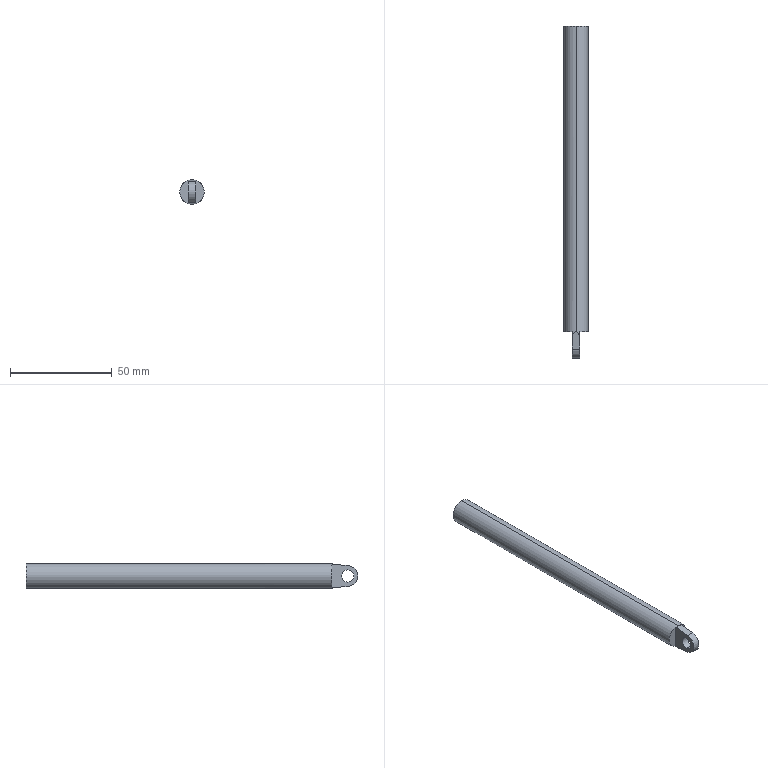Part | SolidWorks | features ICE 2, Extrusion 1, Shell 1 | 1 solid | 15 faces | box 12 x 163 x 12 mm | volume 9872 mm3 | plane 8 | cylinder 7 | commonest cylinder face diameters 6 x2 8 x2 12 x2 10 x1
STEP:
#1=CARTESIAN_POINT('',(1.75,-8.,3.));
#2=VERTEX_POINT('',#1);
#3=CARTESIAN_POINT('',(1.75,-8.,-3.));
#4=VERTEX_POINT('',#3);
#5=CARTESIAN_POINT('',(1.75,-8.,0.));
#6=DIRECTION('',(1.,0.,0.));
#7=DIRECTION('',(0.,0.,-1.));
#8=AXIS2_PLACEMENT_3D('',#5,#6,#7);
#9=CIRCLE('',#8,3.);
#10=EDGE_CURVE('',#2,#4,#9,.T.);
#11=ORIENTED_EDGE('',*,*,#10,.T.);
#12=CARTESIAN_POINT('',(-1.75,-8.,-3.));
#13=VERTEX_POINT('',#12);
#14=CARTESIAN_POINT('',(1.75,-8.,-3.));
#15=DIRECTION('',(-1.,0.,0.));
#16=VECTOR('',#15,1000.);
#17=LINE('',#14,#16);
#18=EDGE_CURVE('',#4,#13,#17,.T.);
#19=ORIENTED_EDGE('',*,*,#18,.T.);
#20=CARTESIAN_POINT('',(-1.75,-8.,3.));
#21=VERTEX_POINT('',#20);
#22=CARTESIAN_POINT('',(-1.75,-8.,0.));
#23=DIRECTION('',(1.,0.,0.));
#24=DIRECTION('',(0.,0.,-1.));
#25=AXIS2_PLACEMENT_3D('',#22,#23,#24);
#26=CIRCLE('',#25,3.);
#27=EDGE_CURVE('',#21,#13,#26,.T.);
#28=ORIENTED_EDGE('',*,*,#27,.F.);
#29=CARTESIAN_POINT('',(1.75,-8.,3.));
#30=DIRECTION('',(-1.,0.,0.));
#31=VECTOR('',#30,1000.);
#32=LINE('',#29,#31);
#33=EDGE_CURVE('',#2,#21,#32,.T.);
#34=ORIENTED_EDGE('',*,*,#33,.F.);
#35=EDGE_LOOP('',(#11,#19,#28,#34));
#36=FACE_OUTER_BOUND('',#35,.T.);
#37=CARTESIAN_POINT('',(1.75,-8.,0.));
#38=DIRECTION('',(-1.,0.,0.));
#39=DIRECTION('',(0.,0.,1.));
#40=AXIS2_PLACEMENT_3D('',#37,#38,#39);
#41=CYLINDRICAL_SURFACE('',#40,3.);
#42=ADVANCED_FACE('',(#36),#41,.F.);
#43=CARTESIAN_POINT('',(0.,150.,-4.));
#44=VERTEX_POINT('',#43);
#45=CARTESIAN_POINT('',(0.,150.,4.));
#46=VERTEX_POINT('',#45);
#47=CARTESIAN_POINT('',(0.,150.,0.));
#48=DIRECTION('',(0.,1.,0.));
#49=DIRECTION('',(0.,0.,1.));
#50=AXIS2_PLACEMENT_3D('',#47,#48,#49);
#51=CIRCLE('',#50,4.);
#52=EDGE_CURVE('',#44,#46,#51,.T.);
#53=ORIENTED_EDGE('',*,*,#52,.T.);
#54=CARTESIAN_POINT('',(0.,2.,4.));
#55=VERTEX_POINT('',#54);
#56=CARTESIAN_POINT('',(0.,150.,4.));
#57=DIRECTION('',(0.,-1.,0.));
#58=VECTOR('',#57,1000.);
#59=LINE('',#56,#58);
#60=EDGE_CURVE('',#46,#55,#59,.T.);
#61=ORIENTED_EDGE('',*,*,#60,.T.);
#62=CARTESIAN_POINT('',(0.,2.,-4.));
#63=VERTEX_POINT('',#62);
#64=CARTESIAN_POINT('',(0.,2.,0.));
#65=DIRECTION('',(0.,1.,0.));
#66=DIRECTION('',(0.,0.,1.));
#67=AXIS2_PLACEMENT_3D('',#64,#65,#66);
#68=CIRCLE('',#67,4.);
#69=EDGE_CURVE('',#63,#55,#68,.T.);
#70=ORIENTED_EDGE('',*,*,#69,.F.);
#71=CARTESIAN_POINT('',(0.,150.,-4.));
#72=DIRECTION('',(0.,-1.,0.));
#73=VECTOR('',#72,1000.);
#74=LINE('',#71,#73);
#75=EDGE_CURVE('',#44,#63,#74,.T.);
#76=ORIENTED_EDGE('',*,*,#75,.F.);
#77=EDGE_LOOP('',(#53,#61,#70,#76));
#78=FACE_OUTER_BOUND('',#77,.T.);
#79=CARTESIAN_POINT('',(0.,150.,0.));
#80=DIRECTION('',(0.,-1.,0.));
#81=DIRECTION('',(0.,0.,-1.));
#82=AXIS2_PLACEMENT_3D('',#79,#80,#81);
#83=CYLINDRICAL_SURFACE('',#82,4.);
#84=ADVANCED_FACE('',(#78),#83,.F.);
#85=CARTESIAN_POINT('',(0.,150.,6.));
#86=VERTEX_POINT('',#85);
#87=CARTESIAN_POINT('',(0.,150.,-6.));
#88=VERTEX_POINT('',#87);
#89=CARTESIAN_POINT('',(0.,150.,0.));
#90=DIRECTION('',(0.,1.,0.));
#91=DIRECTION('',(0.,0.,1.));
#92=AXIS2_PLACEMENT_3D('',#89,#90,#91);
#93=CIRCLE('',#92,6.);
#94=EDGE_CURVE('',#86,#88,#93,.T.);
#95=ORIENTED_EDGE('',*,*,#94,.F.);
#96=CARTESIAN_POINT('',(0.,0.,6.));
#97=VERTEX_POINT('',#96);
#98=CARTESIAN_POINT('',(0.,150.,6.));
#99=DIRECTION('',(0.,-1.,0.));
#100=VECTOR('',#99,1000.);
#101=LINE('',#98,#100);
#102=EDGE_CURVE('',#86,#97,#101,.T.);
#103=ORIENTED_EDGE('',*,*,#102,.T.);
#104=CARTESIAN_POINT('',(1.75,-2.165,5.739));
#105=VERTEX_POINT('',#104);
#106=CARTESIAN_POINT('',(1.75,-2.165,5.739));
#107=CARTESIAN_POINT('',(1.182,-0.7271,5.912));
#108=CARTESIAN_POINT('',(0.5941,0.,6.));
#109=CARTESIAN_POINT('',(0.,0.,6.));
#110=(BOUNDED_CURVE()B_SPLINE_CURVE(3,(#106,#107,#108,#109),.UNSPECIFIED.,.F.,.F.)B_SPLINE_CURVE_WITH_KNOTS((4,4),(5.987,6.283),.UNSPECIFIED.)CURVE()GEOMETRIC_REPRESENTATION_ITEM()RATIONAL_B_SPLINE_CURVE((1.,0.9927,0.9927,1.))REPRESENTATION_ITEM(''));
#111=EDGE_CURVE('',#105,#97,#110,.T.);
#112=ORIENTED_EDGE('',*,*,#111,.F.);
#113=CARTESIAN_POINT('',(1.75,0.,5.739));
#114=VERTEX_POINT('',#113);
#115=CARTESIAN_POINT('',(1.75,-10.,5.739));
#116=DIRECTION('',(0.,1.,0.));
#117=VECTOR('',#116,1000.);
#118=LINE('',#115,#117);
#119=EDGE_CURVE('',#105,#114,#118,.T.);
#120=ORIENTED_EDGE('',*,*,#119,.T.);
#121=CARTESIAN_POINT('',(1.75,0.,-5.739));
#122=VERTEX_POINT('',#121);
#123=CARTESIAN_POINT('',(0.,0.,0.));
#124=DIRECTION('',(0.,1.,0.));
#125=DIRECTION('',(0.,0.,1.));
#126=AXIS2_PLACEMENT_3D('',#123,#124,#125);
#127=CIRCLE('',#126,6.);
#128=EDGE_CURVE('',#114,#122,#127,.T.);
#129=ORIENTED_EDGE('',*,*,#128,.T.);
#130=CARTESIAN_POINT('',(1.75,-2.165,-5.739));
#131=VERTEX_POINT('',#130);
#132=CARTESIAN_POINT('',(1.75,-10.,-5.739));
#133=DIRECTION('',(0.,-1.,0.));
#134=VECTOR('',#133,1000.);
#135=LINE('',#132,#134);
#136=EDGE_CURVE('',#122,#131,#135,.T.);
#137=ORIENTED_EDGE('',*,*,#136,.T.);
#138=CARTESIAN_POINT('',(0.,0.,-6.));
#139=VERTEX_POINT('',#138);
#140=CARTESIAN_POINT('',(0.,0.,-6.));
#141=CARTESIAN_POINT('',(0.5941,0.,-6.));
#142=CARTESIAN_POINT('',(1.182,-0.7271,-5.912));
#143=CARTESIAN_POINT('',(1.75,-2.165,-5.739));
#144=(BOUNDED_CURVE()B_SPLINE_CURVE(3,(#140,#141,#142,#143),.UNSPECIFIED.,.F.,.F.)B_SPLINE_CURVE_WITH_KNOTS((4,4),(0.,0.296),.UNSPECIFIED.)CURVE()GEOMETRIC_REPRESENTATION_ITEM()RATIONAL_B_SPLINE_CURVE((1.,0.9927,0.9927,1.))REPRESENTATION_ITEM(''));
#145=EDGE_CURVE('',#139,#131,#144,.T.);
#146=ORIENTED_EDGE('',*,*,#145,.F.);
#147=CARTESIAN_POINT('',(0.,150.,-6.));
#148=DIRECTION('',(0.,-1.,0.));
#149=VECTOR('',#148,1000.);
#150=LINE('',#147,#149);
#151=EDGE_CURVE('',#88,#139,#150,.T.);
#152=ORIENTED_EDGE('',*,*,#151,.F.);
#153=EDGE_LOOP('',(#95,#103,#112,#120,#129,#137,#146,#152));
#154=FACE_OUTER_BOUND('',#153,.T.);
#155=CARTESIAN_POINT('',(0.,150.,0.));
#156=DIRECTION('',(0.,-1.,0.));
#157=DIRECTION('',(0.,0.,-1.));
#158=AXIS2_PLACEMENT_3D('',#155,#156,#157);
#159=CYLINDRICAL_SURFACE('',#158,6.);
#160=ADVANCED_FACE('',(#154),#159,.T.);
#161=CARTESIAN_POINT('',(1.75,-8.598,4.964));
#162=VERTEX_POINT('',#161);
#163=CARTESIAN_POINT('',(1.75,0.,6.));
#164=DIRECTION('',(0.,-0.9928,-0.1196));
#165=VECTOR('',#164,1000.);
#166=LINE('',#163,#165);
#167=EDGE_CURVE('',#105,#162,#166,.T.);
#168=ORIENTED_EDGE('',*,*,#167,.F.);
#169=ORIENTED_EDGE('',*,*,#111,.T.);
#170=CARTESIAN_POINT('',(-1.75,-2.165,5.739));
#171=VERTEX_POINT('',#170);
#172=CARTESIAN_POINT('',(0.,0.,6.));
#173=CARTESIAN_POINT('',(-0.5941,0.,6.));
#174=CARTESIAN_POINT('',(-1.182,-0.7271,5.912));
#175=CARTESIAN_POINT('',(-1.75,-2.165,5.739));
#176=(BOUNDED_CURVE()B_SPLINE_CURVE(3,(#172,#173,#174,#175),.UNSPECIFIED.,.F.,.F.)B_SPLINE_CURVE_WITH_KNOTS((4,4),(0.,0.296),.UNSPECIFIED.)CURVE()GEOMETRIC_REPRESENTATION_ITEM()RATIONAL_B_SPLINE_CURVE((1.,0.9927,0.9927,1.))REPRESENTATION_ITEM(''));
#177=EDGE_CURVE('',#97,#171,#176,.T.);
#178=ORIENTED_EDGE('',*,*,#177,.T.);
#179=CARTESIAN_POINT('',(-1.75,-8.598,4.964));
#180=VERTEX_POINT('',#179);
#181=CARTESIAN_POINT('',(-1.75,0.,6.));
#182=DIRECTION('',(0.,-0.9928,-0.1196));
#183=VECTOR('',#182,1000.);
#184=LINE('',#181,#183);
#185=EDGE_CURVE('',#171,#180,#184,.T.);
#186=ORIENTED_EDGE('',*,*,#185,.T.);
#187=CARTESIAN_POINT('',(1.75,-8.598,4.964));
#188=DIRECTION('',(-1.,0.,0.));
#189=VECTOR('',#188,1000.);
#190=LINE('',#187,#189);
#191=EDGE_CURVE('',#162,#180,#190,.T.);
#192=ORIENTED_EDGE('',*,*,#191,.F.);
#193=EDGE_LOOP('',(#168,#169,#178,#186,#192));
#194=FACE_OUTER_BOUND('',#193,.T.);
#195=CARTESIAN_POINT('',(1.75,0.,6.));
#196=DIRECTION('',(0.,0.1196,-0.9928));
#197=DIRECTION('',(0.,0.9928,0.1196));
#198=AXIS2_PLACEMENT_3D('',#195,#196,#197);
#199=PLANE('',#198);
#200=ADVANCED_FACE('',(#194),#199,.F.);
#201=CARTESIAN_POINT('',(-1.75,-2.165,-5.739));
#202=VERTEX_POINT('',#201);
#203=CARTESIAN_POINT('',(-1.75,-2.165,-5.739));
#204=CARTESIAN_POINT('',(-1.182,-0.7271,-5.912));
#205=CARTESIAN_POINT('',(-0.5941,0.,-6.));
#206=CARTESIAN_POINT('',(0.,0.,-6.));
#207=(BOUNDED_CURVE()B_SPLINE_CURVE(3,(#203,#204,#205,#206),.UNSPECIFIED.,.F.,.F.)B_SPLINE_CURVE_WITH_KNOTS((4,4),(5.987,6.283),.UNSPECIFIED.)CURVE()GEOMETRIC_REPRESENTATION_ITEM()RATIONAL_B_SPLINE_CURVE((1.,0.9927,0.9927,1.))REPRESENTATION_ITEM(''));
#208=EDGE_CURVE('',#202,#139,#207,.T.);
#209=ORIENTED_EDGE('',*,*,#208,.T.);
#210=ORIENTED_EDGE('',*,*,#145,.T.);
#211=CARTESIAN_POINT('',(1.75,-8.598,-4.964));
#212=VERTEX_POINT('',#211);
#213=CARTESIAN_POINT('',(1.75,0.,-6.));
#214=DIRECTION('',(0.,0.9928,-0.1196));
#215=VECTOR('',#214,1000.);
#216=LINE('',#213,#215);
#217=EDGE_CURVE('',#212,#131,#216,.T.);
#218=ORIENTED_EDGE('',*,*,#217,.F.);
#219=CARTESIAN_POINT('',(-1.75,-8.598,-4.964));
#220=VERTEX_POINT('',#219);
#221=CARTESIAN_POINT('',(1.75,-8.598,-4.964));
#222=DIRECTION('',(-1.,0.,0.));
#223=VECTOR('',#222,1000.);
#224=LINE('',#221,#223);
#225=EDGE_CURVE('',#212,#220,#224,.T.);
#226=ORIENTED_EDGE('',*,*,#225,.T.);
#227=CARTESIAN_POINT('',(-1.75,0.,-6.));
#228=DIRECTION('',(0.,0.9928,-0.1196));
#229=VECTOR('',#228,1000.);
#230=LINE('',#227,#229);
#231=EDGE_CURVE('',#220,#202,#230,.T.);
#232=ORIENTED_EDGE('',*,*,#231,.T.);
#233=EDGE_LOOP('',(#209,#210,#218,#226,#232));
#234=FACE_OUTER_BOUND('',#233,.T.);
#235=CARTESIAN_POINT('',(1.75,0.,-6.));
#236=DIRECTION('',(0.,0.1196,0.9928));
#237=DIRECTION('',(0.,-0.9928,0.1196));
#238=AXIS2_PLACEMENT_3D('',#235,#236,#237);
#239=PLANE('',#238);
#240=ADVANCED_FACE('',(#234),#239,.F.);
#241=CARTESIAN_POINT('',(1.75,0.,6.));
#242=DIRECTION('',(0.,0.,1.));
#243=VECTOR('',#242,1000.);
#244=LINE('',#241,#243);
#245=EDGE_CURVE('',#122,#114,#244,.T.);
#246=ORIENTED_EDGE('',*,*,#245,.F.);
#247=ORIENTED_EDGE('',*,*,#128,.F.);
#248=EDGE_LOOP('',(#246,#247));
#249=FACE_OUTER_BOUND('',#248,.T.);
#250=CARTESIAN_POINT('',(0.,0.,0.));
#251=DIRECTION('',(0.,1.,0.));
#252=DIRECTION('',(0.,0.,1.));
#253=AXIS2_PLACEMENT_3D('',#250,#251,#252);
#254=PLANE('',#253);
#255=ADVANCED_FACE('',(#249),#254,.F.);
#256=ORIENTED_EDGE('',*,*,#102,.F.);
#257=CARTESIAN_POINT('',(0.,150.,0.));
#258=DIRECTION('',(0.,1.,0.));
#259=DIRECTION('',(0.,0.,1.));
#260=AXIS2_PLACEMENT_3D('',#257,#258,#259);
#261=CIRCLE('',#260,6.);
#262=EDGE_CURVE('',#88,#86,#261,.T.);
#263=ORIENTED_EDGE('',*,*,#262,.F.);
#264=ORIENTED_EDGE('',*,*,#151,.T.);
#265=ORIENTED_EDGE('',*,*,#208,.F.);
#266=CARTESIAN_POINT('',(-1.75,0.,-5.739));
#267=VERTEX_POINT('',#266);
#268=CARTESIAN_POINT('',(-1.75,-10.,-5.739));
#269=DIRECTION('',(0.,-1.,0.));
#270=VECTOR('',#269,1000.);
#271=LINE('',#268,#270);
#272=EDGE_CURVE('',#267,#202,#271,.T.);
#273=ORIENTED_EDGE('',*,*,#272,.F.);
#274=CARTESIAN_POINT('',(-1.75,0.,5.739));
#275=VERTEX_POINT('',#274);
#276=CARTESIAN_POINT('',(0.,0.,0.));
#277=DIRECTION('',(0.,1.,0.));
#278=DIRECTION('',(0.,0.,1.));
#279=AXIS2_PLACEMENT_3D('',#276,#277,#278);
#280=CIRCLE('',#279,6.);
#281=EDGE_CURVE('',#267,#275,#280,.T.);
#282=ORIENTED_EDGE('',*,*,#281,.T.);
#283=CARTESIAN_POINT('',(-1.75,-10.,5.739));
#284=DIRECTION('',(0.,1.,0.));
#285=VECTOR('',#284,1000.);
#286=LINE('',#283,#285);
#287=EDGE_CURVE('',#171,#275,#286,.T.);
#288=ORIENTED_EDGE('',*,*,#287,.F.);
#289=ORIENTED_EDGE('',*,*,#177,.F.);
#290=EDGE_LOOP('',(#256,#263,#264,#265,#273,#282,#288,#289));
#291=FACE_OUTER_BOUND('',#290,.T.);
#292=CARTESIAN_POINT('',(0.,150.,0.));
#293=DIRECTION('',(0.,-1.,0.));
#294=DIRECTION('',(0.,0.,-1.));
#295=AXIS2_PLACEMENT_3D('',#292,#293,#294);
#296=CYLINDRICAL_SURFACE('',#295,6.);
#297=ADVANCED_FACE('',(#291),#296,.T.);
#298=ORIENTED_EDGE('',*,*,#52,.F.);
#299=CARTESIAN_POINT('',(0.,150.,0.));
#300=DIRECTION('',(0.,1.,0.));
#301=DIRECTION('',(0.,0.,1.));
#302=AXIS2_PLACEMENT_3D('',#299,#300,#301);
#303=CIRCLE('',#302,4.);
#304=EDGE_CURVE('',#46,#44,#303,.T.);
#305=ORIENTED_EDGE('',*,*,#304,.F.);
#306=EDGE_LOOP('',(#298,#305));
#307=FACE_BOUND('',#306,.T.);
#308=ORIENTED_EDGE('',*,*,#262,.T.);
#309=ORIENTED_EDGE('',*,*,#94,.T.);
#310=EDGE_LOOP('',(#308,#309));
#311=FACE_OUTER_BOUND('',#310,.T.);
#312=CARTESIAN_POINT('',(0.,150.,0.));
#313=DIRECTION('',(0.,1.,0.));
#314=DIRECTION('',(0.,0.,1.));
#315=AXIS2_PLACEMENT_3D('',#312,#313,#314);
#316=PLANE('',#315);
#317=ADVANCED_FACE('',(#307,#311),#316,.T.);
#318=ORIENTED_EDGE('',*,*,#281,.F.);
#319=CARTESIAN_POINT('',(-1.75,0.,6.));
#320=DIRECTION('',(0.,0.,1.));
#321=VECTOR('',#320,1000.);
#322=LINE('',#319,#321);
#323=EDGE_CURVE('',#267,#275,#322,.T.);
#324=ORIENTED_EDGE('',*,*,#323,.T.);
#325=EDGE_LOOP('',(#318,#324));
#326=FACE_OUTER_BOUND('',#325,.T.);
#327=CARTESIAN_POINT('',(0.,0.,0.));
#328=DIRECTION('',(0.,1.,0.));
#329=DIRECTION('',(0.,0.,1.));
#330=AXIS2_PLACEMENT_3D('',#327,#328,#329);
#331=PLANE('',#330);
#332=ADVANCED_FACE('',(#326),#331,.F.);
#333=ORIENTED_EDGE('',*,*,#60,.F.);
#334=ORIENTED_EDGE('',*,*,#304,.T.);
#335=ORIENTED_EDGE('',*,*,#75,.T.);
#336=CARTESIAN_POINT('',(0.,2.,0.));
#337=DIRECTION('',(0.,1.,0.));
#338=DIRECTION('',(0.,0.,1.));
#339=AXIS2_PLACEMENT_3D('',#336,#337,#338);
#340=CIRCLE('',#339,4.);
#341=EDGE_CURVE('',#55,#63,#340,.T.);
#342=ORIENTED_EDGE('',*,*,#341,.F.);
#343=EDGE_LOOP('',(#333,#334,#335,#342));
#344=FACE_OUTER_BOUND('',#343,.T.);
#345=CARTESIAN_POINT('',(0.,150.,0.));
#346=DIRECTION('',(0.,-1.,0.));
#347=DIRECTION('',(0.,0.,-1.));
#348=AXIS2_PLACEMENT_3D('',#345,#346,#347);
#349=CYLINDRICAL_SURFACE('',#348,4.);
#350=ADVANCED_FACE('',(#344),#349,.F.);
#351=ORIENTED_EDGE('',*,*,#69,.T.);
#352=ORIENTED_EDGE('',*,*,#341,.T.);
#353=EDGE_LOOP('',(#351,#352));
#354=FACE_OUTER_BOUND('',#353,.T.);
#355=CARTESIAN_POINT('',(0.,2.,0.));
#356=DIRECTION('',(0.,1.,0.));
#357=DIRECTION('',(0.,0.,1.));
#358=AXIS2_PLACEMENT_3D('',#355,#356,#357);
#359=PLANE('',#358);
#360=ADVANCED_FACE('',(#354),#359,.T.);
#361=ORIENTED_EDGE('',*,*,#136,.F.);
#362=ORIENTED_EDGE('',*,*,#245,.T.);
#363=ORIENTED_EDGE('',*,*,#119,.F.);
#364=ORIENTED_EDGE('',*,*,#167,.T.);
#365=CARTESIAN_POINT('',(1.75,-8.,0.));
#366=DIRECTION('',(1.,0.,0.));
#367=DIRECTION('',(0.,0.,-1.));
#368=AXIS2_PLACEMENT_3D('',#365,#366,#367);
#369=CIRCLE('',#368,5.);
#370=EDGE_CURVE('',#162,#212,#369,.T.);
#371=ORIENTED_EDGE('',*,*,#370,.T.);
#372=ORIENTED_EDGE('',*,*,#217,.T.);
#373=EDGE_LOOP('',(#361,#362,#363,#364,#371,#372));
#374=FACE_OUTER_BOUND('',#373,.T.);
#375=ORIENTED_EDGE('',*,*,#10,.F.);
#376=CARTESIAN_POINT('',(1.75,-8.,0.));
#377=DIRECTION('',(1.,0.,0.));
#378=DIRECTION('',(0.,0.,-1.));
#379=AXIS2_PLACEMENT_3D('',#376,#377,#378);
#380=CIRCLE('',#379,3.);
#381=EDGE_CURVE('',#4,#2,#380,.T.);
#382=ORIENTED_EDGE('',*,*,#381,.F.);
#383=EDGE_LOOP('',(#375,#382));
#384=FACE_BOUND('',#383,.T.);
#385=CARTESIAN_POINT('',(1.75,-8.,0.));
#386=DIRECTION('',(1.,0.,0.));
#387=DIRECTION('',(0.,0.,-1.));
#388=AXIS2_PLACEMENT_3D('',#385,#386,#387);
#389=PLANE('',#388);
#390=ADVANCED_FACE('',(#374,#384),#389,.T.);
#391=ORIENTED_EDGE('',*,*,#323,.F.);
#392=ORIENTED_EDGE('',*,*,#272,.T.);
#393=ORIENTED_EDGE('',*,*,#231,.F.);
#394=CARTESIAN_POINT('',(-1.75,-8.,0.));
#395=DIRECTION('',(1.,0.,0.));
#396=DIRECTION('',(0.,0.,-1.));
#397=AXIS2_PLACEMENT_3D('',#394,#395,#396);
#398=CIRCLE('',#397,5.);
#399=EDGE_CURVE('',#180,#220,#398,.T.);
#400=ORIENTED_EDGE('',*,*,#399,.F.);
#401=ORIENTED_EDGE('',*,*,#185,.F.);
#402=ORIENTED_EDGE('',*,*,#287,.T.);
#403=EDGE_LOOP('',(#391,#392,#393,#400,#401,#402));
#404=FACE_OUTER_BOUND('',#403,.T.);
#405=ORIENTED_EDGE('',*,*,#27,.T.);
#406=CARTESIAN_POINT('',(-1.75,-8.,0.));
#407=DIRECTION('',(1.,0.,0.));
#408=DIRECTION('',(0.,0.,-1.));
#409=AXIS2_PLACEMENT_3D('',#406,#407,#408);
#410=CIRCLE('',#409,3.);
#411=EDGE_CURVE('',#13,#21,#410,.T.);
#412=ORIENTED_EDGE('',*,*,#411,.T.);
#413=EDGE_LOOP('',(#405,#412));
#414=FACE_BOUND('',#413,.T.);
#415=CARTESIAN_POINT('',(-1.75,-8.,0.));
#416=DIRECTION('',(1.,0.,0.));
#417=DIRECTION('',(0.,0.,-1.));
#418=AXIS2_PLACEMENT_3D('',#415,#416,#417);
#419=PLANE('',#418);
#420=ADVANCED_FACE('',(#404,#414),#419,.F.);
#421=ORIENTED_EDGE('',*,*,#399,.T.);
#422=ORIENTED_EDGE('',*,*,#225,.F.);
#423=ORIENTED_EDGE('',*,*,#370,.F.);
#424=ORIENTED_EDGE('',*,*,#191,.T.);
#425=EDGE_LOOP('',(#421,#422,#423,#424));
#426=FACE_OUTER_BOUND('',#425,.T.);
#427=CARTESIAN_POINT('',(1.75,-8.,0.));
#428=DIRECTION('',(-1.,0.,0.));
#429=DIRECTION('',(0.,0.,1.));
#430=AXIS2_PLACEMENT_3D('',#427,#428,#429);
#431=CYLINDRICAL_SURFACE('',#430,5.);
#432=ADVANCED_FACE('',(#426),#431,.T.);
#433=ORIENTED_EDGE('',*,*,#18,.F.);
#434=ORIENTED_EDGE('',*,*,#381,.T.);
#435=ORIENTED_EDGE('',*,*,#33,.T.);
#436=ORIENTED_EDGE('',*,*,#411,.F.);
#437=EDGE_LOOP('',(#433,#434,#435,#436));
#438=FACE_OUTER_BOUND('',#437,.T.);
#439=CARTESIAN_POINT('',(1.75,-8.,0.));
#440=DIRECTION('',(-1.,0.,0.));
#441=DIRECTION('',(0.,0.,1.));
#442=AXIS2_PLACEMENT_3D('',#439,#440,#441);
#443=CYLINDRICAL_SURFACE('',#442,3.);
#444=ADVANCED_FACE('',(#438),#443,.F.);
#445=CLOSED_SHELL('',(#42,#84,#160,#200,#240,#255,#297,#317,#332,#350,#360,#390,#420,#432,#444));
#446=MANIFOLD_SOLID_BREP('',#445);
#447=CARTESIAN_POINT('',(0.,0.,0.));
#448=DIRECTION('',(0.,0.,1.));
#449=DIRECTION('',(1.,0.,0.));
#450=AXIS2_PLACEMENT_3D('',#447,#448,#449);
#451=(LENGTH_UNIT()NAMED_UNIT(*)SI_UNIT(.MILLI.,.METRE.));
#452=UNCERTAINTY_MEASURE_WITH_UNIT(LENGTH_MEASURE(0.00001),#451,'','');
#453=(NAMED_UNIT(*)PLANE_ANGLE_UNIT()SI_UNIT($,.RADIAN.));
#454=(NAMED_UNIT(*)SI_UNIT($,.STERADIAN.)SOLID_ANGLE_UNIT());
#455=(GEOMETRIC_REPRESENTATION_CONTEXT(3)GLOBAL_UNCERTAINTY_ASSIGNED_CONTEXT((#452))GLOBAL_UNIT_ASSIGNED_CONTEXT((#451,#453,#454))REPRESENTATION_CONTEXT('',''));
#456=ADVANCED_BREP_SHAPE_REPRESENTATION('',(#446,#450),#455);